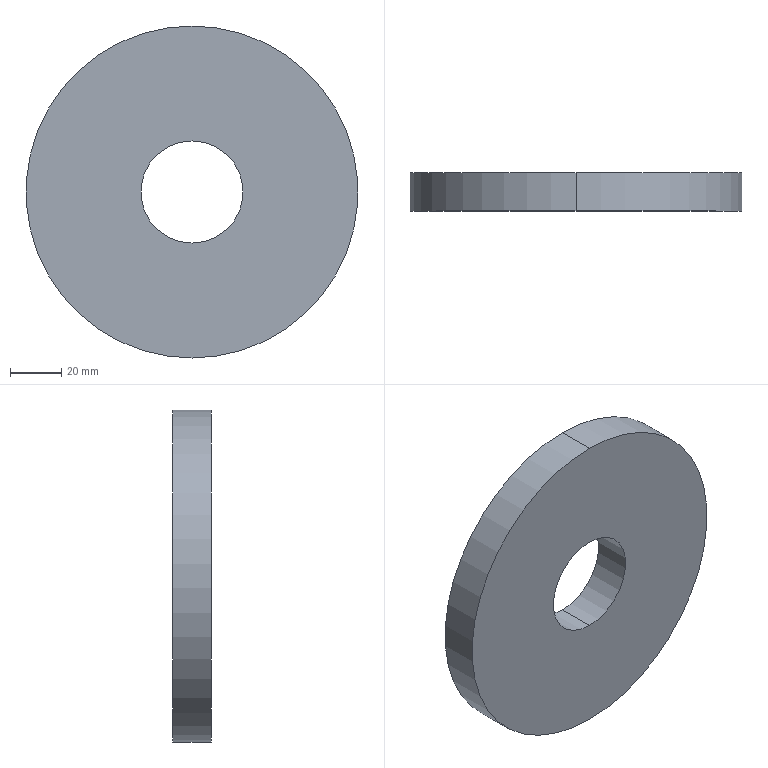Part | SolidWorks | features Extrusion 1 | 1 solid | 6 faces | box 130 x 15 x 130 mm | volume 180249 mm3 | cylinder 4 | plane 2 | commonest cylinder face diameters 40 x2 130 x2
STEP:
#1=CARTESIAN_POINT('',(0.,7.5,-20.));
#2=VERTEX_POINT('',#1);
#3=CARTESIAN_POINT('',(0.,7.5,20.));
#4=VERTEX_POINT('',#3);
#5=CARTESIAN_POINT('',(0.,7.5,0.));
#6=DIRECTION('',(0.,1.,0.));
#7=DIRECTION('',(0.,0.,1.));
#8=AXIS2_PLACEMENT_3D('',#5,#6,#7);
#9=CIRCLE('',#8,20.);
#10=EDGE_CURVE('',#2,#4,#9,.T.);
#11=ORIENTED_EDGE('',*,*,#10,.T.);
#12=CARTESIAN_POINT('',(0.,-7.5,20.));
#13=VERTEX_POINT('',#12);
#14=CARTESIAN_POINT('',(0.,7.5,20.));
#15=DIRECTION('',(0.,-1.,0.));
#16=VECTOR('',#15,1000.);
#17=LINE('',#14,#16);
#18=EDGE_CURVE('',#4,#13,#17,.T.);
#19=ORIENTED_EDGE('',*,*,#18,.T.);
#20=CARTESIAN_POINT('',(0.,-7.5,-20.));
#21=VERTEX_POINT('',#20);
#22=CARTESIAN_POINT('',(0.,-7.5,0.));
#23=DIRECTION('',(0.,1.,0.));
#24=DIRECTION('',(0.,0.,1.));
#25=AXIS2_PLACEMENT_3D('',#22,#23,#24);
#26=CIRCLE('',#25,20.);
#27=EDGE_CURVE('',#21,#13,#26,.T.);
#28=ORIENTED_EDGE('',*,*,#27,.F.);
#29=CARTESIAN_POINT('',(0.,7.5,-20.));
#30=DIRECTION('',(0.,-1.,0.));
#31=VECTOR('',#30,1000.);
#32=LINE('',#29,#31);
#33=EDGE_CURVE('',#2,#21,#32,.T.);
#34=ORIENTED_EDGE('',*,*,#33,.F.);
#35=EDGE_LOOP('',(#11,#19,#28,#34));
#36=FACE_OUTER_BOUND('',#35,.T.);
#37=CARTESIAN_POINT('',(0.,7.5,0.));
#38=DIRECTION('',(0.,-1.,0.));
#39=DIRECTION('',(0.,0.,-1.));
#40=AXIS2_PLACEMENT_3D('',#37,#38,#39);
#41=CYLINDRICAL_SURFACE('',#40,20.);
#42=ADVANCED_FACE('',(#36),#41,.F.);
#43=CARTESIAN_POINT('',(0.,7.5,65.));
#44=VERTEX_POINT('',#43);
#45=CARTESIAN_POINT('',(0.,7.5,-65.));
#46=VERTEX_POINT('',#45);
#47=CARTESIAN_POINT('',(0.,7.5,0.));
#48=DIRECTION('',(0.,1.,0.));
#49=DIRECTION('',(0.,0.,1.));
#50=AXIS2_PLACEMENT_3D('',#47,#48,#49);
#51=CIRCLE('',#50,65.);
#52=EDGE_CURVE('',#44,#46,#51,.T.);
#53=ORIENTED_EDGE('',*,*,#52,.F.);
#54=CARTESIAN_POINT('',(0.,-7.5,65.));
#55=VERTEX_POINT('',#54);
#56=CARTESIAN_POINT('',(0.,7.5,65.));
#57=DIRECTION('',(0.,-1.,0.));
#58=VECTOR('',#57,1000.);
#59=LINE('',#56,#58);
#60=EDGE_CURVE('',#44,#55,#59,.T.);
#61=ORIENTED_EDGE('',*,*,#60,.T.);
#62=CARTESIAN_POINT('',(0.,-7.5,-65.));
#63=VERTEX_POINT('',#62);
#64=CARTESIAN_POINT('',(0.,-7.5,0.));
#65=DIRECTION('',(0.,1.,0.));
#66=DIRECTION('',(0.,0.,1.));
#67=AXIS2_PLACEMENT_3D('',#64,#65,#66);
#68=CIRCLE('',#67,65.);
#69=EDGE_CURVE('',#55,#63,#68,.T.);
#70=ORIENTED_EDGE('',*,*,#69,.T.);
#71=CARTESIAN_POINT('',(0.,7.5,-65.));
#72=DIRECTION('',(0.,-1.,0.));
#73=VECTOR('',#72,1000.);
#74=LINE('',#71,#73);
#75=EDGE_CURVE('',#46,#63,#74,.T.);
#76=ORIENTED_EDGE('',*,*,#75,.F.);
#77=EDGE_LOOP('',(#53,#61,#70,#76));
#78=FACE_OUTER_BOUND('',#77,.T.);
#79=CARTESIAN_POINT('',(0.,7.5,0.));
#80=DIRECTION('',(0.,-1.,0.));
#81=DIRECTION('',(0.,0.,-1.));
#82=AXIS2_PLACEMENT_3D('',#79,#80,#81);
#83=CYLINDRICAL_SURFACE('',#82,65.);
#84=ADVANCED_FACE('',(#78),#83,.T.);
#85=CARTESIAN_POINT('',(0.,7.5,0.));
#86=DIRECTION('',(0.,1.,0.));
#87=DIRECTION('',(0.,0.,1.));
#88=AXIS2_PLACEMENT_3D('',#85,#86,#87);
#89=CIRCLE('',#88,65.);
#90=EDGE_CURVE('',#46,#44,#89,.T.);
#91=ORIENTED_EDGE('',*,*,#90,.T.);
#92=ORIENTED_EDGE('',*,*,#52,.T.);
#93=EDGE_LOOP('',(#91,#92));
#94=FACE_OUTER_BOUND('',#93,.T.);
#95=ORIENTED_EDGE('',*,*,#10,.F.);
#96=CARTESIAN_POINT('',(0.,7.5,0.));
#97=DIRECTION('',(0.,1.,0.));
#98=DIRECTION('',(0.,0.,1.));
#99=AXIS2_PLACEMENT_3D('',#96,#97,#98);
#100=CIRCLE('',#99,20.);
#101=EDGE_CURVE('',#4,#2,#100,.T.);
#102=ORIENTED_EDGE('',*,*,#101,.F.);
#103=EDGE_LOOP('',(#95,#102));
#104=FACE_BOUND('',#103,.T.);
#105=CARTESIAN_POINT('',(0.,7.5,0.));
#106=DIRECTION('',(0.,1.,0.));
#107=DIRECTION('',(0.,0.,1.));
#108=AXIS2_PLACEMENT_3D('',#105,#106,#107);
#109=PLANE('',#108);
#110=ADVANCED_FACE('',(#94,#104),#109,.T.);
#111=CARTESIAN_POINT('',(0.,-7.5,0.));
#112=DIRECTION('',(0.,1.,0.));
#113=DIRECTION('',(0.,0.,1.));
#114=AXIS2_PLACEMENT_3D('',#111,#112,#113);
#115=CIRCLE('',#114,65.);
#116=EDGE_CURVE('',#63,#55,#115,.T.);
#117=ORIENTED_EDGE('',*,*,#116,.F.);
#118=ORIENTED_EDGE('',*,*,#69,.F.);
#119=EDGE_LOOP('',(#117,#118));
#120=FACE_OUTER_BOUND('',#119,.T.);
#121=ORIENTED_EDGE('',*,*,#27,.T.);
#122=CARTESIAN_POINT('',(0.,-7.5,0.));
#123=DIRECTION('',(0.,1.,0.));
#124=DIRECTION('',(0.,0.,1.));
#125=AXIS2_PLACEMENT_3D('',#122,#123,#124);
#126=CIRCLE('',#125,20.);
#127=EDGE_CURVE('',#13,#21,#126,.T.);
#128=ORIENTED_EDGE('',*,*,#127,.T.);
#129=EDGE_LOOP('',(#121,#128));
#130=FACE_BOUND('',#129,.T.);
#131=CARTESIAN_POINT('',(0.,-7.5,0.));
#132=DIRECTION('',(0.,1.,0.));
#133=DIRECTION('',(0.,0.,1.));
#134=AXIS2_PLACEMENT_3D('',#131,#132,#133);
#135=PLANE('',#134);
#136=ADVANCED_FACE('',(#120,#130),#135,.F.);
#137=ORIENTED_EDGE('',*,*,#60,.F.);
#138=ORIENTED_EDGE('',*,*,#90,.F.);
#139=ORIENTED_EDGE('',*,*,#75,.T.);
#140=ORIENTED_EDGE('',*,*,#116,.T.);
#141=EDGE_LOOP('',(#137,#138,#139,#140));
#142=FACE_OUTER_BOUND('',#141,.T.);
#143=CARTESIAN_POINT('',(0.,7.5,0.));
#144=DIRECTION('',(0.,-1.,0.));
#145=DIRECTION('',(0.,0.,-1.));
#146=AXIS2_PLACEMENT_3D('',#143,#144,#145);
#147=CYLINDRICAL_SURFACE('',#146,65.);
#148=ADVANCED_FACE('',(#142),#147,.T.);
#149=ORIENTED_EDGE('',*,*,#18,.F.);
#150=ORIENTED_EDGE('',*,*,#101,.T.);
#151=ORIENTED_EDGE('',*,*,#33,.T.);
#152=ORIENTED_EDGE('',*,*,#127,.F.);
#153=EDGE_LOOP('',(#149,#150,#151,#152));
#154=FACE_OUTER_BOUND('',#153,.T.);
#155=CARTESIAN_POINT('',(0.,7.5,0.));
#156=DIRECTION('',(0.,-1.,0.));
#157=DIRECTION('',(0.,0.,-1.));
#158=AXIS2_PLACEMENT_3D('',#155,#156,#157);
#159=CYLINDRICAL_SURFACE('',#158,20.);
#160=ADVANCED_FACE('',(#154),#159,.F.);
#161=CLOSED_SHELL('',(#42,#84,#110,#136,#148,#160));
#162=MANIFOLD_SOLID_BREP('',#161);
#163=CARTESIAN_POINT('',(0.,0.,0.));
#164=DIRECTION('',(0.,0.,1.));
#165=DIRECTION('',(1.,0.,0.));
#166=AXIS2_PLACEMENT_3D('',#163,#164,#165);
#167=(LENGTH_UNIT()NAMED_UNIT(*)SI_UNIT(.MILLI.,.METRE.));
#168=UNCERTAINTY_MEASURE_WITH_UNIT(LENGTH_MEASURE(0.00001),#167,'','');
#169=(NAMED_UNIT(*)PLANE_ANGLE_UNIT()SI_UNIT($,.RADIAN.));
#170=(NAMED_UNIT(*)SI_UNIT($,.STERADIAN.)SOLID_ANGLE_UNIT());
#171=(GEOMETRIC_REPRESENTATION_CONTEXT(3)GLOBAL_UNCERTAINTY_ASSIGNED_CONTEXT((#168))GLOBAL_UNIT_ASSIGNED_CONTEXT((#167,#169,#170))REPRESENTATION_CONTEXT('',''));
#172=ADVANCED_BREP_SHAPE_REPRESENTATION('',(#162,#166),#171);